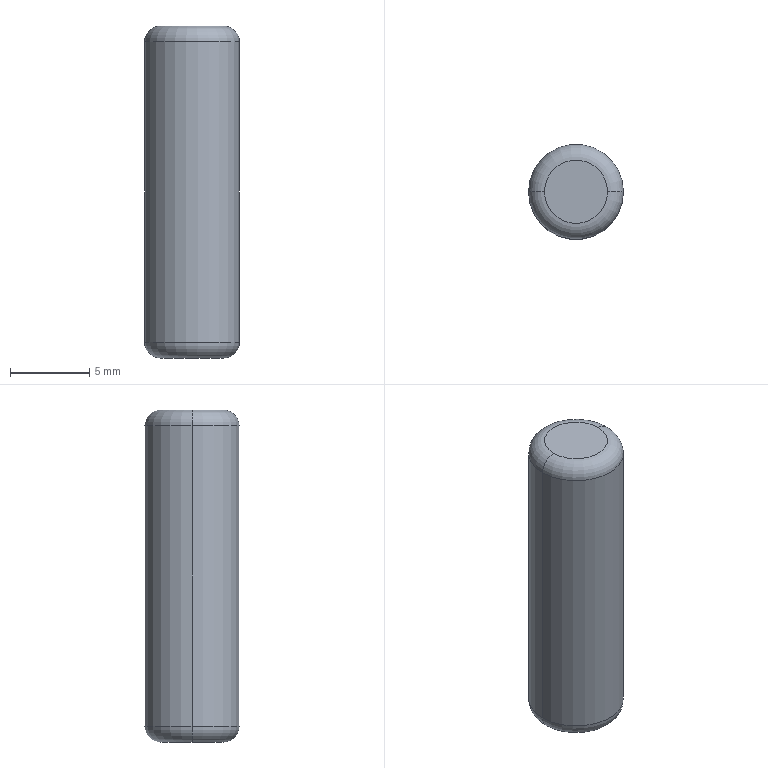Part | SolidWorks | features Extrusion 1, Fillet 1 | 1 solid | 8 faces | box 6 x 6 x 21 mm | volume 586.273 mm3 | torus 4 | cylinder 2 | plane 2 | commonest cylinder face diameters 6 x2
STEP:
#1=CARTESIAN_POINT('',(-3.,0.,20.));
#2=VERTEX_POINT('',#1);
#3=CARTESIAN_POINT('',(3.,0.,20.));
#4=VERTEX_POINT('',#3);
#5=CARTESIAN_POINT('',(0.,0.,20.));
#6=DIRECTION('',(0.,0.,-1.));
#7=DIRECTION('',(1.,0.,0.));
#8=AXIS2_PLACEMENT_3D('',#5,#6,#7);
#9=CIRCLE('',#8,3.);
#10=EDGE_CURVE('',#2,#4,#9,.T.);
#11=ORIENTED_EDGE('',*,*,#10,.F.);
#12=CARTESIAN_POINT('',(-2.,0.,21.));
#13=VERTEX_POINT('',#12);
#14=CARTESIAN_POINT('',(-2.,0.,20.));
#15=DIRECTION('',(0.,1.,0.));
#16=DIRECTION('',(-1.,0.,0.));
#17=AXIS2_PLACEMENT_3D('',#14,#15,#16);
#18=CIRCLE('',#17,1.);
#19=EDGE_CURVE('',#2,#13,#18,.T.);
#20=ORIENTED_EDGE('',*,*,#19,.T.);
#21=CARTESIAN_POINT('',(2.,0.,21.));
#22=VERTEX_POINT('',#21);
#23=CARTESIAN_POINT('',(0.,0.,21.));
#24=DIRECTION('',(0.,0.,1.));
#25=DIRECTION('',(1.,0.,0.));
#26=AXIS2_PLACEMENT_3D('',#23,#24,#25);
#27=CIRCLE('',#26,2.);
#28=EDGE_CURVE('',#22,#13,#27,.T.);
#29=ORIENTED_EDGE('',*,*,#28,.F.);
#30=CARTESIAN_POINT('',(2.,0.,20.));
#31=DIRECTION('',(0.,-1.,0.));
#32=DIRECTION('',(0.,0.,-1.));
#33=AXIS2_PLACEMENT_3D('',#30,#31,#32);
#34=CIRCLE('',#33,1.);
#35=EDGE_CURVE('',#4,#22,#34,.T.);
#36=ORIENTED_EDGE('',*,*,#35,.F.);
#37=EDGE_LOOP('',(#11,#20,#29,#36));
#38=FACE_OUTER_BOUND('',#37,.T.);
#39=CARTESIAN_POINT('',(0.,0.,20.));
#40=DIRECTION('',(0.,0.,1.));
#41=DIRECTION('',(1.,0.,0.));
#42=AXIS2_PLACEMENT_3D('',#39,#40,#41);
#43=TOROIDAL_SURFACE('',#42,2.,1.);
#44=ADVANCED_FACE('',(#38),#43,.T.);
#45=CARTESIAN_POINT('',(-2.,0.,0.));
#46=VERTEX_POINT('',#45);
#47=CARTESIAN_POINT('',(2.,0.,0.));
#48=VERTEX_POINT('',#47);
#49=CARTESIAN_POINT('',(0.,0.,0.));
#50=DIRECTION('',(0.,0.,-1.));
#51=DIRECTION('',(1.,0.,0.));
#52=AXIS2_PLACEMENT_3D('',#49,#50,#51);
#53=CIRCLE('',#52,2.);
#54=EDGE_CURVE('',#46,#48,#53,.T.);
#55=ORIENTED_EDGE('',*,*,#54,.F.);
#56=CARTESIAN_POINT('',(-3.,0.,1.));
#57=VERTEX_POINT('',#56);
#58=CARTESIAN_POINT('',(-2.,0.,1.));
#59=DIRECTION('',(0.,1.,0.));
#60=DIRECTION('',(-1.,0.,0.));
#61=AXIS2_PLACEMENT_3D('',#58,#59,#60);
#62=CIRCLE('',#61,1.);
#63=EDGE_CURVE('',#46,#57,#62,.T.);
#64=ORIENTED_EDGE('',*,*,#63,.T.);
#65=CARTESIAN_POINT('',(3.,0.,1.));
#66=VERTEX_POINT('',#65);
#67=CARTESIAN_POINT('',(0.,0.,1.));
#68=DIRECTION('',(0.,0.,1.));
#69=DIRECTION('',(1.,0.,0.));
#70=AXIS2_PLACEMENT_3D('',#67,#68,#69);
#71=CIRCLE('',#70,3.);
#72=EDGE_CURVE('',#66,#57,#71,.T.);
#73=ORIENTED_EDGE('',*,*,#72,.F.);
#74=CARTESIAN_POINT('',(2.,0.,1.));
#75=DIRECTION('',(0.,-1.,0.));
#76=DIRECTION('',(0.,0.,-1.));
#77=AXIS2_PLACEMENT_3D('',#74,#75,#76);
#78=CIRCLE('',#77,1.);
#79=EDGE_CURVE('',#48,#66,#78,.T.);
#80=ORIENTED_EDGE('',*,*,#79,.F.);
#81=EDGE_LOOP('',(#55,#64,#73,#80));
#82=FACE_OUTER_BOUND('',#81,.T.);
#83=CARTESIAN_POINT('',(0.,0.,1.));
#84=DIRECTION('',(0.,0.,1.));
#85=DIRECTION('',(1.,0.,0.));
#86=AXIS2_PLACEMENT_3D('',#83,#84,#85);
#87=TOROIDAL_SURFACE('',#86,2.,1.);
#88=ADVANCED_FACE('',(#82),#87,.T.);
#89=ORIENTED_EDGE('',*,*,#10,.T.);
#90=CARTESIAN_POINT('',(3.,0.,21.));
#91=DIRECTION('',(0.,0.,-1.));
#92=VECTOR('',#91,1000.);
#93=LINE('',#90,#92);
#94=EDGE_CURVE('',#4,#66,#93,.T.);
#95=ORIENTED_EDGE('',*,*,#94,.T.);
#96=ORIENTED_EDGE('',*,*,#72,.T.);
#97=CARTESIAN_POINT('',(-3.,0.,21.));
#98=DIRECTION('',(0.,0.,-1.));
#99=VECTOR('',#98,1000.);
#100=LINE('',#97,#99);
#101=EDGE_CURVE('',#2,#57,#100,.T.);
#102=ORIENTED_EDGE('',*,*,#101,.F.);
#103=EDGE_LOOP('',(#89,#95,#96,#102));
#104=FACE_OUTER_BOUND('',#103,.T.);
#105=CARTESIAN_POINT('',(0.,0.,21.));
#106=DIRECTION('',(0.,0.,-1.));
#107=DIRECTION('',(-1.,0.,0.));
#108=AXIS2_PLACEMENT_3D('',#105,#106,#107);
#109=CYLINDRICAL_SURFACE('',#108,3.);
#110=ADVANCED_FACE('',(#104),#109,.T.);
#111=ORIENTED_EDGE('',*,*,#94,.F.);
#112=CARTESIAN_POINT('',(0.,0.,20.));
#113=DIRECTION('',(0.,0.,-1.));
#114=DIRECTION('',(1.,0.,0.));
#115=AXIS2_PLACEMENT_3D('',#112,#113,#114);
#116=CIRCLE('',#115,3.);
#117=EDGE_CURVE('',#4,#2,#116,.T.);
#118=ORIENTED_EDGE('',*,*,#117,.T.);
#119=ORIENTED_EDGE('',*,*,#101,.T.);
#120=CARTESIAN_POINT('',(0.,0.,1.));
#121=DIRECTION('',(0.,0.,1.));
#122=DIRECTION('',(1.,0.,0.));
#123=AXIS2_PLACEMENT_3D('',#120,#121,#122);
#124=CIRCLE('',#123,3.);
#125=EDGE_CURVE('',#57,#66,#124,.T.);
#126=ORIENTED_EDGE('',*,*,#125,.T.);
#127=EDGE_LOOP('',(#111,#118,#119,#126));
#128=FACE_OUTER_BOUND('',#127,.T.);
#129=CARTESIAN_POINT('',(0.,0.,21.));
#130=DIRECTION('',(0.,0.,-1.));
#131=DIRECTION('',(-1.,0.,0.));
#132=AXIS2_PLACEMENT_3D('',#129,#130,#131);
#133=CYLINDRICAL_SURFACE('',#132,3.);
#134=ADVANCED_FACE('',(#128),#133,.T.);
#135=ORIENTED_EDGE('',*,*,#28,.T.);
#136=CARTESIAN_POINT('',(0.,0.,21.));
#137=DIRECTION('',(0.,0.,1.));
#138=DIRECTION('',(1.,0.,0.));
#139=AXIS2_PLACEMENT_3D('',#136,#137,#138);
#140=CIRCLE('',#139,2.);
#141=EDGE_CURVE('',#13,#22,#140,.T.);
#142=ORIENTED_EDGE('',*,*,#141,.T.);
#143=EDGE_LOOP('',(#135,#142));
#144=FACE_OUTER_BOUND('',#143,.T.);
#145=CARTESIAN_POINT('',(0.,0.,21.));
#146=DIRECTION('',(0.,0.,1.));
#147=DIRECTION('',(1.,0.,0.));
#148=AXIS2_PLACEMENT_3D('',#145,#146,#147);
#149=PLANE('',#148);
#150=ADVANCED_FACE('',(#144),#149,.T.);
#151=CARTESIAN_POINT('',(0.,0.,0.));
#152=DIRECTION('',(0.,0.,-1.));
#153=DIRECTION('',(1.,0.,0.));
#154=AXIS2_PLACEMENT_3D('',#151,#152,#153);
#155=CIRCLE('',#154,2.);
#156=EDGE_CURVE('',#48,#46,#155,.T.);
#157=ORIENTED_EDGE('',*,*,#156,.T.);
#158=ORIENTED_EDGE('',*,*,#54,.T.);
#159=EDGE_LOOP('',(#157,#158));
#160=FACE_OUTER_BOUND('',#159,.T.);
#161=CARTESIAN_POINT('',(0.,0.,0.));
#162=DIRECTION('',(0.,0.,1.));
#163=DIRECTION('',(1.,0.,0.));
#164=AXIS2_PLACEMENT_3D('',#161,#162,#163);
#165=PLANE('',#164);
#166=ADVANCED_FACE('',(#160),#165,.F.);
#167=ORIENTED_EDGE('',*,*,#63,.F.);
#168=ORIENTED_EDGE('',*,*,#156,.F.);
#169=ORIENTED_EDGE('',*,*,#79,.T.);
#170=ORIENTED_EDGE('',*,*,#125,.F.);
#171=EDGE_LOOP('',(#167,#168,#169,#170));
#172=FACE_OUTER_BOUND('',#171,.T.);
#173=CARTESIAN_POINT('',(0.,0.,1.));
#174=DIRECTION('',(0.,0.,1.));
#175=DIRECTION('',(1.,0.,0.));
#176=AXIS2_PLACEMENT_3D('',#173,#174,#175);
#177=TOROIDAL_SURFACE('',#176,2.,1.);
#178=ADVANCED_FACE('',(#172),#177,.T.);
#179=ORIENTED_EDGE('',*,*,#19,.F.);
#180=ORIENTED_EDGE('',*,*,#117,.F.);
#181=ORIENTED_EDGE('',*,*,#35,.T.);
#182=ORIENTED_EDGE('',*,*,#141,.F.);
#183=EDGE_LOOP('',(#179,#180,#181,#182));
#184=FACE_OUTER_BOUND('',#183,.T.);
#185=CARTESIAN_POINT('',(0.,0.,20.));
#186=DIRECTION('',(0.,0.,1.));
#187=DIRECTION('',(1.,0.,0.));
#188=AXIS2_PLACEMENT_3D('',#185,#186,#187);
#189=TOROIDAL_SURFACE('',#188,2.,1.);
#190=ADVANCED_FACE('',(#184),#189,.T.);
#191=CLOSED_SHELL('',(#44,#88,#110,#134,#150,#166,#178,#190));
#192=MANIFOLD_SOLID_BREP('',#191);
#193=CARTESIAN_POINT('',(0.,0.,0.));
#194=DIRECTION('',(0.,0.,1.));
#195=DIRECTION('',(1.,0.,0.));
#196=AXIS2_PLACEMENT_3D('',#193,#194,#195);
#197=(LENGTH_UNIT()NAMED_UNIT(*)SI_UNIT(.MILLI.,.METRE.));
#198=UNCERTAINTY_MEASURE_WITH_UNIT(LENGTH_MEASURE(0.00001),#197,'','');
#199=(NAMED_UNIT(*)PLANE_ANGLE_UNIT()SI_UNIT($,.RADIAN.));
#200=(NAMED_UNIT(*)SI_UNIT($,.STERADIAN.)SOLID_ANGLE_UNIT());
#201=(GEOMETRIC_REPRESENTATION_CONTEXT(3)GLOBAL_UNCERTAINTY_ASSIGNED_CONTEXT((#198))GLOBAL_UNIT_ASSIGNED_CONTEXT((#197,#199,#200))REPRESENTATION_CONTEXT('',''));
#202=ADVANCED_BREP_SHAPE_REPRESENTATION('',(#192,#196),#201);